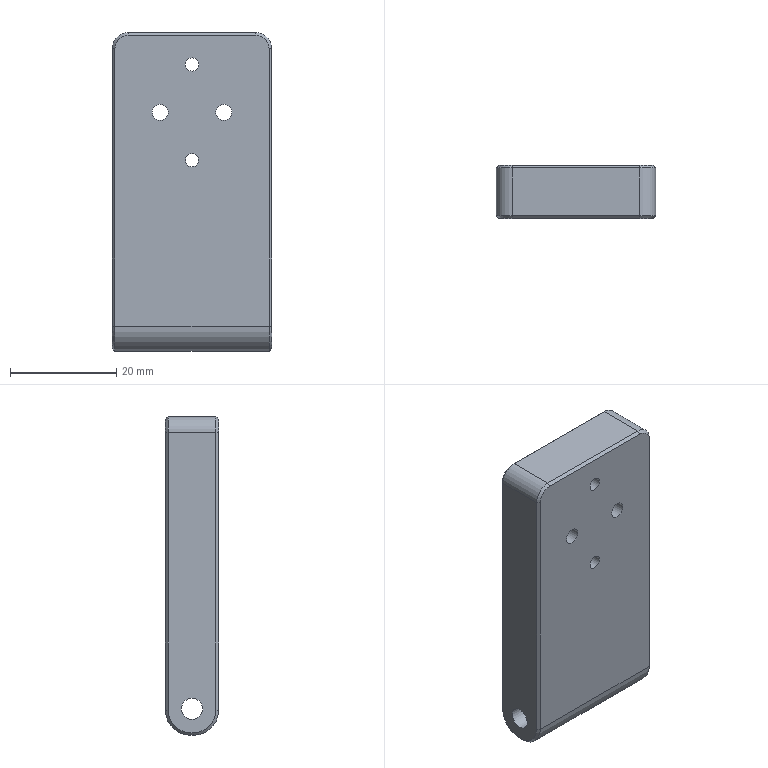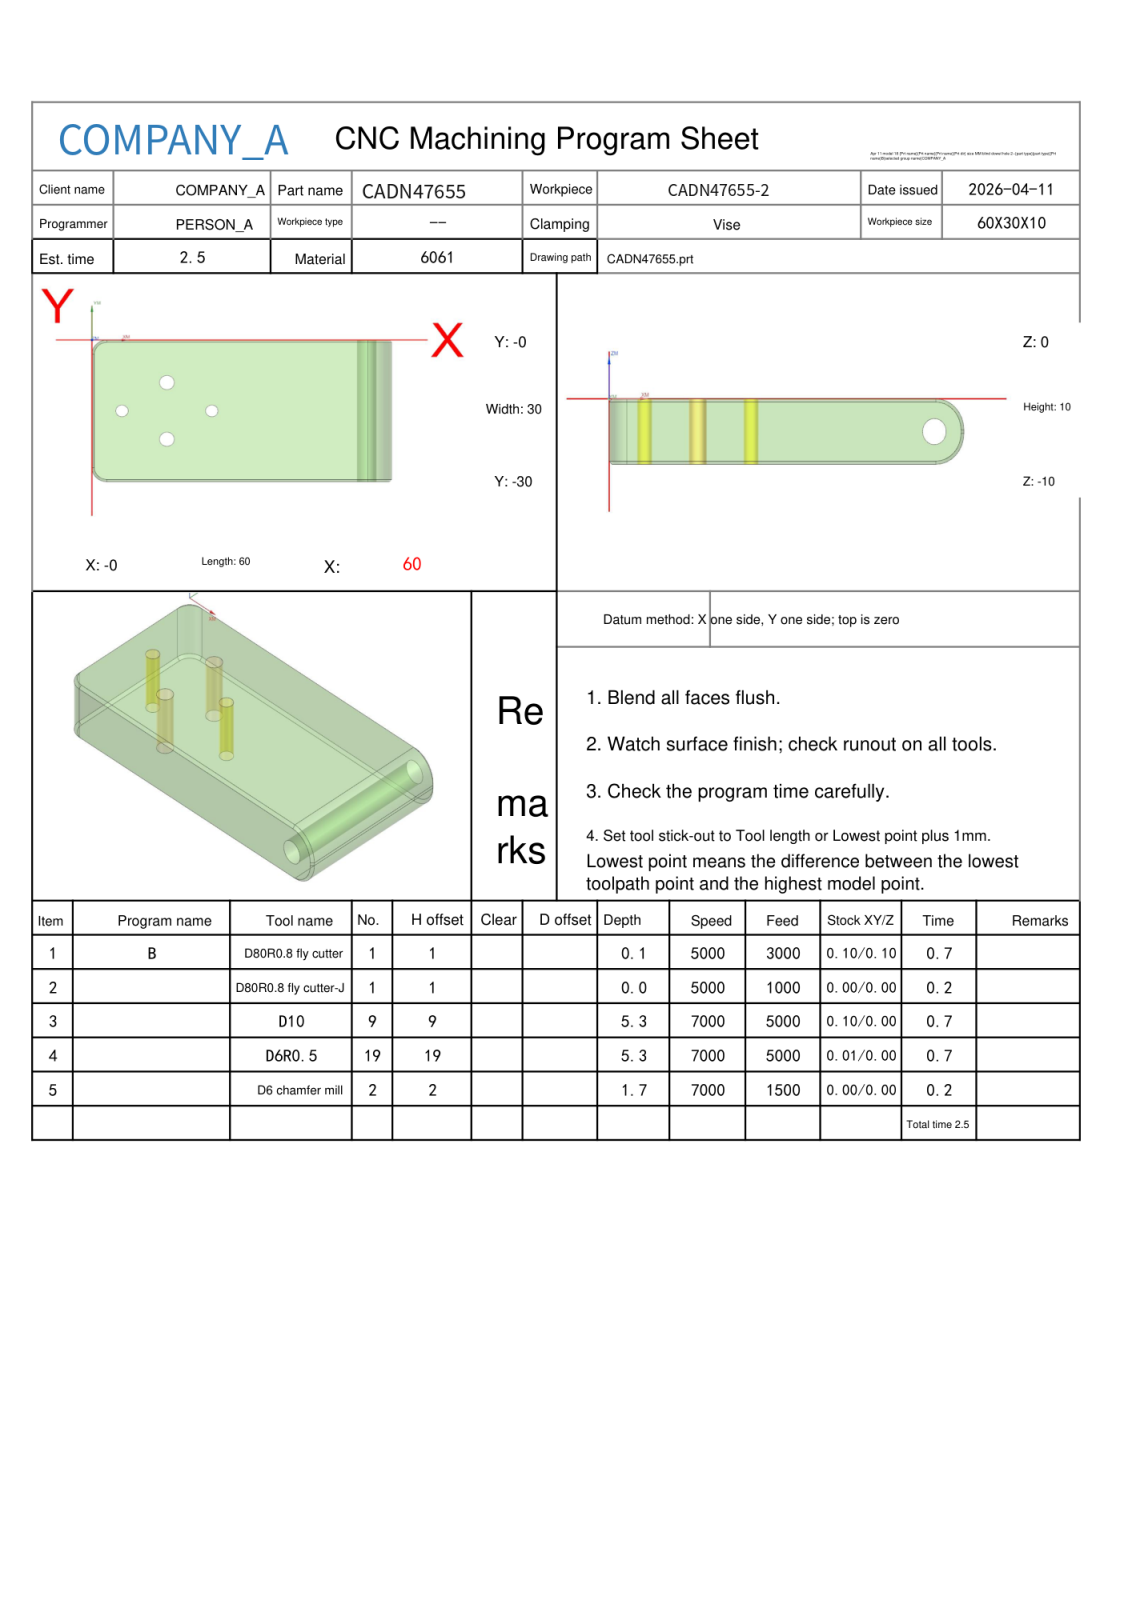NC program | NX | posted by the shop | part box 30 x 10 x 60 mm
Whole program, first 1498 of 1636 lines:
%
O0001
(Machine time: 3.37 MIN)
(===Total Tool:4===)
(T1=D80R0.8 fly cutter D=80.  R=0.8  D-  H01 Z=-0.   )
(T9=D10     D=10.  R=0.   D-  H09 Z=-5.35 )
(T19=D6R0.5 D=6.   R=0.5  D-  H19 Z=-5.35 )
(T2=D6 chamfer mill   D=6.   R=0.   D-  H02 Z=-1.75 )
G80 G90 G17 G49 G40
G91 G28 Z0
M01
N1 T01 M06
(D80R0.8 fly cutter  D=80. R=0.8 H=01 ce=0.10 di=0.10)
G00 G90 G54 X112.097 Y-15. M03 S5000
G43 H01 Z20.
M08
Z6.011
G01 Z4.011 F3000.
X100.097
X-40.097
X-52.097
Z6.011
G00 X112.097
Z5.522
G01 Z3.522
X100.097
X-40.097
X-52.097
Z5.522
G00 X112.097
Z5.033
G01 Z3.033
X100.097
X-40.097
X-52.097
Z5.033
G00 X112.097
Z4.544
G01 Z2.544
X100.097
X-40.097
X-52.097
Z4.544
G00 Z20.
X112.097
Z4.056
G01 Z2.056
X100.097
X-40.097
X-52.097
Z4.056
G00 Z20.
X112.097
Z3.567
G01 Z1.567
X100.097
X-40.097
X-52.097
Z3.567
G00 Z20.
X112.097
Z3.078
G01 Z1.078
X100.097
X-40.097
X-52.097
Z3.078
G00 Z20.
X112.097
Z2.589
G01 Z.589
X100.097
X-40.097
X-52.097
Z2.589
G00 Z20.
X112.097
Z2.1
G01 Z.1
X100.097
X-40.097
X-52.097
Z2.1
G00 Z20.
G91 G28 Z0.0
M05
M09
G91 G28 Z0.0
M01
N2 T01 M06
(D80R0.8 fly cutter-J  D=80. R=0.8 H=01 ce=0.00 di=0.00)
G00 G90 G54 X111.999 Y-14.998 M03 S5000
G43 H01 Z20.
M08
Z2.
G01 Z0.0 F1000.
X99.999 Y-14.999
X-39.999 Y-15.002
X-51.999
Z2.
G00 Z20.
G91 G28 Z0.0
M05
M09
G91 G28 Z0.0
M01
N3 T09 M06
(D10  D=10. R=0. H=09 ce=0.10 di=0.00)
G00 G90 G54 X48.978 Y9.606 M03 S7000
G43 H09 Z11.8
M08
Z.494
G01 Z-.006 F5000.
X48.983 Y9.445
G03 X53.98 Y4.604 I4.997 J.159
G01 X54.139 Y4.606
G02 X54.681 Y4.615 I.542 J-17.03
X56.195 Y4.548 I0.0 J-17.038
X60.598 Y-.5 I-.804 J-5.146
G01 Y-29.5
G02 X56.195 Y-34.548 I-5.208 J.098
X54.735 Y-34.618 I-1.46 J15.079
X54.139 Y-34.606 I0.0 J15.15
G01 X54.14 Y-34.614 Z-.014
G03 X54.692 Y-34.621 I.552 J22.478
X55.975 Y-34.584 I0.0 J22.485
X60.717 Y-29.5 I-.431 J5.155
G01 Y-.5
G03 X56.195 Y4.557 I-5.124 J-.031
X54.738 Y4.626 I-1.457 J-15.541
X54.14 Y4.614 I0.0 J-15.609
G01 Y4.624 Z-.024
G02 X54.724 Y4.632 I.584 J-21.478
X55.88 Y4.601 I0.0 J-21.485
X60.828 Y-.5 I-.243 J-5.186
G01 Y-29.5
G02 X55.976 Y-34.596 I-5.192 J.085
X54.688 Y-34.63 I-1.288 J23.89
X54.14 Y-34.624 I0.0 J23.925
G01 Y-34.636 Z-.036
G03 X54.7 Y-34.643 I.56 J21.788
X56.059 Y-34.601 I0.0 J21.795
X60.935 Y-29.5 I-.297 J5.165
G01 Y-.5
G03 X56.036 Y4.601 I-5.171 J-.063
X54.735 Y4.645 I-1.301 J-18.968
X54.14 Y4.636 I0.0 J-19.012
G01 Y4.65 Z-.05
G02 X54.742 Y4.66 I.602 J-18.398
X56.389 Y4.586 I0.0 J-18.408
X61.039 Y-.5 I-.457 J-5.086
G01 Y-29.5
G02 X56.195 Y-34.603 I-5.161 J.049
X54.715 Y-34.659 I-1.479 J19.52
X54.14 Y-34.65 I0.0 J19.576
G01 X54.141 Y-34.667 Z-.067
G03 X54.732 Y-34.677 I.591 J17.174
X56.588 Y-34.576 I0.0 J17.185
X61.142 Y-29.5 I-.551 J5.076
G01 Y-.5
G03 X56.64 Y4.567 I-5.154 J-.046
G01 X56.344 Y4.601
G03 X54.754 Y4.678 I-1.59 J-16.378
X54.141 Y4.667 I0.0 J-16.455
G01 Y4.685 Z-.085
G02 X54.768 Y4.697 I.626 J-15.524
X56.64 Y4.584 I0.0 J-15.536
X61.244 Y-.5 I-.562 J-5.135
G01 Y-29.5
G02 X56.64 Y-34.584 I-5.166 J.051
X54.753 Y-34.697 I-1.887 J15.791
X54.141 Y-34.685 I0.0 J15.903
G01 X54.142 Y-34.705 Z-.105
G03 X54.66 Y-34.709 I.518 J31.553
X55.75 Y-34.691 I0.0 J31.557
X57.606 Y-34.401 I-.349 J8.339
X61.344 Y-29.502 I-1.342 J4.9
G01 Y-.472
G03 X60.729 Y1.897 I-4.869 J0.0
X56.64 Y4.604 I-4.657 J-2.593
X54.77 Y4.718 I-1.87 J-15.236
X54.142 Y4.705 I0.0 J-15.35
G01 Y4.728 Z-.128
G02 X54.738 Y4.737 I.596 J-18.49
X56.195 Y4.68 I0.0 J-18.499
X58.419 Y4.157 I-.658 J-7.794
X61.444 Y-.5 I-2.142 J-4.702
G01 Y-29.5
G02 X57.084 Y-34.549 I-5.142 J.034
X54.782 Y-34.742 I-2.302 J13.584
X54.142 Y-34.728 I0.0 J13.777
G01 X54.143 Y-34.752 Z-.152
G03 X54.783 Y-34.767 I.64 J13.742
X56.914 Y-34.601 I0.0 J13.757
G01 X57.084 Y-34.572
X57.529 Y-34.483
G03 X61.542 Y-29.5 I-1.129 J5.017
G01 Y-.498
G03 X57.748 Y4.424 I-5.089 J0.0
X55.75 Y4.737 I-2.528 J-9.609
X54.718 Y4.759 I-1.032 J-24.001
X54.143 Y4.752 I0.0 J-24.023
G01 X54.144 Y4.779 Z-.179
X55.305 Y4.778
G02 X57.974 Y4.392 I-.124 J-10.256
X61.64 Y-.5 I-1.477 J-4.927
G01 Y-29.5
G02 X57.974 Y-34.392 I-5.143 J.035
G01 X57.794 Y-34.44
G02 X55.202 Y-34.778 I-2.595 J9.768
G01 X54.143 Y-34.779
X54.144 Y-34.807 Z-.207
X55.305
G03 X58.154 Y-34.362 I-.097 J9.96
X61.737 Y-29.502 I-1.505 J4.86
G01 Y-.5
G03 X58.16 Y4.36 I-5.09 J0.0
X55.75 Y4.791 I-2.92 J-9.382
X54.719 Y4.814 I-1.031 J-22.682
X54.144 Y4.807 I0.0 J-22.705
G01 X54.145 Y4.838 Z-.238
G02 X54.72 Y4.845 I.574 J-22.026
X55.75 Y4.821 I0.0 J-22.034
X58.441 Y4.294 I-.46 J-9.473
X61.834 Y-.498 I-1.688 J-4.792
G01 Y-29.503
G02 X58.315 Y-34.343 I-5.088 J0.0
X55.305 Y-34.837 I-3.131 J9.652
G01 X54.145 Y-34.838
Y-34.87 Z-.27
X55.305
G03 X58.559 Y-34.288 I-.102 J9.957
X61.929 Y-29.502 I-1.713 J4.786
G01 Y-.499
G03 X58.567 Y4.286 I-5.085 J0.0
X55.75 Y4.853 I-3.328 J-9.243
X54.72 Y4.878 I-1.03 J-21.336
X54.146 Y4.87 I0.0 J-21.36
G01 X54.147 Y4.905 Z-.305
G02 X54.729 Y4.914 I.582 J-18.707
X55.764 Y4.885 I0.0 J-18.716
X58.686 Y4.282 I-.559 J-10.094
X62.024 Y-.498 I-1.753 J-4.78
G01 Y-29.505
G02 X58.613 Y-34.309 I-5.089 J0.0
X55.104 Y-34.905 I-3.511 J10.056
G01 X54.146
X54.147 Y-34.941 Z-.341
X55.305
G03 X58.863 Y-34.253 I-.168 J10.412
X62.118 Y-29.5 I-1.886 J4.782
G01 Y-.5
G03 X58.863 Y4.253 I-5.14 J-.029
X56.195 Y4.893 I-3.842 J-10.141
X54.727 Y4.95 I-1.468 J-18.704
X54.148 Y4.941 I0.0 J-18.762
G01 X54.149 Y4.98 Z-.38
G02 X54.724 Y4.989 I.576 J-18.802
X56.195 Y4.931 I0.0 J-18.81
X58.863 Y4.289 I-1.197 J-10.845
X62.211 Y-.5 I-1.799 J-4.822
G01 Y-29.5
G02 X58.863 Y-34.289 I-5.146 J.033
X55.305 Y-34.979 I-3.734 J9.729
G01 X54.148 Y-34.98
X54.149 Y-35.02 Z-.42
X55.101
G03 X59.197 Y-34.189 I-.003 J10.526
X62.303 Y-29.503 I-1.981 J4.686
G01 Y-.497
G03 X59.225 Y4.177 I-5.088 J0.0
X55.644 Y5.006 I-4.086 J-9.502
X54.722 Y5.029 I-.922 J-18.84
X54.15 Y5.02 I0.0 J-18.862
G01 X54.152 Y5.062 Z-.462
G02 X54.641 Y5.068 I.489 J-22.187
X56.195 Y5.013 I0.0 J-22.193
X59.308 Y4.184 I-1.24 J-10.912
X62.394 Y-.5 I-2.05 J-4.709
G01 Y-29.5
G02 X59.308 Y-34.184 I-5.136 J.026
X56.195 Y-35.013 I-4.354 J10.084
X54.641 Y-35.068 I-1.554 J22.149
X54.152 Y-35.062 I0.0 J22.203
G01 X54.157 Y-35.085 Z-.485
X54.162 Y-35.106 Z-.507
G03 X54.628 Y-35.11 I.467 J23.01
X56.195 Y-35.057 I0.0 J23.015
X59.753 Y-34.015 I-1.22 J10.758
X62.485 Y-29.5 I-2.416 J4.546
G01 Y-.5
G03 X59.753 Y4.015 I-5.148 J-.031
X56.195 Y5.057 I-4.778 J-9.715
X54.611 Y5.111 I-1.584 J-23.31
X54.162 Y5.106 I0.0 J-23.364
G01 X54.163 Y5.129 Z-.53
X54.164 Y5.15 Z-.553
G02 X54.634 Y5.155 I.47 J-21.914
X56.195 Y5.1 I0.0 J-21.919
X59.753 Y4.06 I-1.224 J-10.799
X62.574 Y-.5 I-2.316 J-4.585
G01 Y-29.5
G02 X59.753 Y-34.06 I-5.137 J.025
X56.195 Y-35.099 I-4.782 J9.759
X54.657 Y-35.155 I-1.538 J21.308
X54.163 Y-35.149 I0.0 J21.363
G01 X54.164 Y-35.175 Z-.577
X54.165 Y-35.197 Z-.601
G03 X54.635 Y-35.202 I.47 J20.915
X56.195 Y-35.144 I0.0 J20.921
X59.928 Y-34.009 I-1.162 J10.529
X62.662 Y-29.501 I-2.349 J4.508
G01 Y-.497
G03 X59.959 Y3.994 I-5.081 J0.0
X55.638 Y5.178 I-4.812 J-9.084
X54.605 Y5.202 I-1.033 J-21.632
X54.166 Y5.198 I0.0 J-21.657
G01 X54.167 Y5.225 Z-.626
X54.168 Y5.247 Z-.65
G02 X54.575 Y5.251 I.407 J-21.392
X56.195 Y5.19 I0.0 J-21.396
X60.082 Y3.975 I-1.168 J-10.564
X62.749 Y-.499 I-2.419 J-4.474
G01 Y-29.501
G02 X60.082 Y-33.975 I-5.086 J0.0
X56.195 Y-35.19 I-5.054 J9.346
X54.613 Y-35.251 I-1.582 J20.422
X54.167 Y-35.246 I0.0 J20.483
G01 X54.168 Y-35.273 Z-.676
X54.169 Y-35.297 Z-.702
G03 X54.591 Y-35.301 I.423 J20.046
X55.655 Y-35.273 I0.0 J20.051
X60.325 Y-33.882 I-.552 J10.389
X62.835 Y-29.523 I-2.53 J4.359
G01 Y-.472
G03 X60.353 Y3.867 I-5.033 J0.0
X55.702 Y5.27 I-5.214 J-8.871
X54.544 Y5.302 I-1.157 J-21.104
X54.169 Y5.299 I0.0 J-21.136
G01 X54.171 Y5.328 Z-.729
X54.172 Y5.352 Z-.755
G02 X54.513 Y5.355 I.342 J-20.874
X55.769 Y5.317 I0.0 J-20.877
X59.918 Y4.15 I-.611 J-10.131
G01 X60.198 Y4.007
G02 X62.92 Y-.5 I-2.389 J-4.519
G01 Y-29.5
G02 X60.198 Y-34.007 I-5.112 J.012
G01 X59.766 Y-34.228
G02 X55.795 Y-35.316 I-4.603 J9.011
X54.57 Y-35.354 I-1.225 J19.587
X54.171 Y-35.35 I0.0 J19.626
G01 X54.172 Y-35.379 Z-.783
X54.173 Y-35.404 Z-.811
G03 X54.548 Y-35.408 I.375 J19.204
X55.805 Y-35.367 I0.0 J19.208
X59.762 Y-34.277 I-.665 J10.136
G01 X60.198 Y-34.054
G03 X63.004 Y-29.5 I-2.303 J4.561
G01 Y-.5
G03 X60.198 Y4.054 I-5.109 J-.007
G01 X60.009 Y4.15
G03 X55.76 Y5.369 I-4.884 J-9.009
X54.482 Y5.409 I-1.278 J-20.581
X54.174 Y5.407 I0.0 J-20.621
G01 X54.175 Y5.437 Z-.839
X54.176 Y5.463 Z-.867
G02 X54.45 Y5.465 I.274 J-20.366
X56.195 Y5.39 I0.0 J-20.368
X60.198 Y4.102 I-1.186 J-10.546
G01 X60.5 Y3.931
G02 X63.086 Y-.495 I-2.496 J-4.427
G01 Y-29.497
G02 X60.494 Y-33.935 I-5.094 J0.0
G01 X60.198 Y-34.102
G02 X56.195 Y-35.39 I-5.186 J9.254
X54.526 Y-35.464 I-1.668 J18.723
X54.175 Y-35.461 I0.0 J18.797
G01 X54.191 Y-35.519 Z-.926
G03 X54.616 Y-35.525 I.425 J14.224
X57.084 Y-35.309 I0.0 J14.23
X60.958 Y-33.7 I-2.338 J11.093
X63.168 Y-29.5 I-2.904 J4.209
G01 Y-.5
G03 X60.958 Y3.7 I-5.113 J-.009
X57.084 Y5.31 I-6.218 J-9.494
X54.575 Y5.527 I-2.51 J-14.406
X54.193 Y5.522 I0.0 J-14.623
G01 X54.237 Y5.582 Z-.986
G02 X54.58 Y5.586 I.343 J-14.294
X57.084 Y5.365 I0.0 J-14.298
X60.951 Y3.753 I-2.387 J-11.174
X63.248 Y-.493 I-2.777 J-4.246
G01 Y-29.508
G02 X60.952 Y-33.753 I-5.073 J0.0
X57.084 Y-35.364 I-6.249 J9.551
X54.609 Y-35.583 I-2.476 J13.88
X54.234 Y-35.578 I0.0 J14.099
G01 X54.279 Y-35.639 Z-1.048
G03 X54.615 Y-35.643 I.336 J13.803
X57.084 Y-35.421 I0.0 J13.807
X60.642 Y-33.997 I-2.388 J11.128
G01 X60.934 Y-33.815
G03 X63.327 Y-29.499 I-2.696 J4.316
G01 Y-.497
G03 X60.937 Y3.813 I-5.082 J0.0
G01 X60.642 Y3.997
G03 X57.084 Y5.421 I-5.953 J-9.715
X54.604 Y5.647 I-2.48 J-13.505
X54.282 Y5.643 I0.0 J-13.731
G01 X54.328 Y5.707 Z-1.112
G02 X54.672 Y5.711 I.345 J-12.45
X57.529 Y5.379 I0.0 J-12.455
X61.194 Y3.7 I-3.171 J-11.757
X63.404 Y-.5 I-2.902 J-4.208
G01 Y-29.5
G02 X61.194 Y-33.7 I-5.112 J.008
X57.529 Y-35.378 I-6.818 J10.046
X54.658 Y-35.706 I-2.871 J12.416
X54.325 Y-35.702 I0.0 J12.744
G01 X54.372 Y-35.765 Z-1.177
G03 X54.645 Y-35.768 I.273 J13.145
X57.084 Y-35.54 I0.0 J13.148
X61.532 Y-33.508 I-2.603 J11.58
X63.48 Y-29.5 I-3.167 J4.017
G01 Y-.5
G03 X61.532 Y3.508 I-5.115 J-.009
X57.529 Y5.438 I-7.159 J-9.727
X54.701 Y5.776 I-2.828 J-11.682
X54.375 Y5.771 I0.0 J-12.019
G01 X54.551 Y5.833 Z-1.244
G02 X54.881 Y5.838 I.33 J-10.415
X58.863 Y5.047 I0.0 J-10.421
G01 X59.143 Y4.928
G02 X61.087 Y3.866 I-4.43 J-10.422
G01 X61.217 Y3.783
G02 X63.555 Y-.495 I-2.744 J-4.278
G01 Y-29.5
G02 X61.346 Y-33.7 I-5.118 J.011
G01 X60.787 Y-34.058
G02 X57.084 Y-35.604 I-6.225 J9.703
X54.747 Y-35.828 I-2.338 J12.08
X54.499 Y-35.826 I0.0 J12.305
G01 X54.705 Y-35.838 Z-1.258
X54.91 Y-35.847 Z-1.271
X55.116 Y-35.856 Z-1.285
X55.322 Y-35.864 Z-1.299
X55.527 Y-35.861 Z-1.312
G03 X57.974 Y-35.434 I-.333 J9.13
X61.087 Y-33.917 I-3.909 J11.975
G01 X61.418 Y-33.7
G03 X63.628 Y-29.5 I-2.897 J4.206
G01 Y-.498
G03 X61.335 Y3.754 I-5.088 J0.0
G01 X61.087 Y3.917
G03 X59.126 Y4.99 I-6.424 J-9.411
G01 X58.982 Y5.052
X58.863 Y5.107
G03 X55.652 Y5.866 I-3.812 J-8.944
G01 X55.867 Z-1.326
X56.082 Y5.86 Z-1.34
X56.297 Y5.85 Z-1.354
X56.511 Y5.83 Z-1.368
X56.723 Y5.805 Z-1.382
G02 X58.48 Y5.322 I-1.474 J-8.797
X61.532 Y3.671 I-5.033 J-12.949
X63.7 Y-.5 I-2.945 J-4.179
G01 Y-29.5
G02 X61.532 Y-33.671 I-5.112 J.008
X58.419 Y-35.345 I-8.076 J11.289
X56.703 Y-35.805 I-3.253 J8.695
G01 X56.893 Y-35.79 Z-1.4
X57.083 Y-35.772 Z-1.418
X57.272 Y-35.746 Z-1.436
X57.458 Y-35.712 Z-1.454
G03 X58.419 Y-35.408 I-2.214 J8.654
X61.786 Y-33.533 I-5.004 J12.948
X63.77 Y-29.5 I-3.122 J4.04
G01 Y-.5
G03 X61.719 Y3.585 I-5.093 J0.0
X58.419 Y5.409 I-8.348 J-11.207
X57.457 Y5.711 I-2.883 J-7.498
G01 X57.64 Y5.686 Z-1.478
X57.821 Y5.655 Z-1.502
X58.002 Y5.622 Z-1.526
G02 X61.632 Y3.7 I-4.521 J-12.926
G01 X61.977 Y3.436
G02 X63.839 Y-.5 I-3.247 J-3.945
G01 Y-29.5
G02 X61.813 Y-33.567 I-5.116 J.011
G01 X61.632 Y-33.7
G02 X57.999 Y-35.622 I-8.146 J11.
G01 X58.21 Y-35.585 Z-1.563
X58.417 Y-35.538 Z-1.601
G03 X61.958 Y-33.504 I-5.321 J13.357
X63.906 Y-29.505 I-3.13 J3.998
G01 Y-.5
G03 X61.977 Y3.492 I-5.109 J-.007
X58.419 Y5.539 I-8.968 J-11.473
G01 X58.603 Y5.499 Z-1.638
X58.787 Y5.457 Z-1.676
G02 X61.977 Y3.539 I-6.175 J-13.886
X63.971 Y-.5 I-3.103 J-4.045
G01 Y-29.504
G02 X62.044 Y-33.487 I-5.078 J0.0
X58.785 Y-35.456 I-9.426 J11.916
G01 X58.939 Y-35.426 Z-1.715
X59.087 Y-35.381 Z-1.753
G03 X62.166 Y-33.436 I-6.578 J13.82
X64.035 Y-29.506 I-3.196 J3.93
G01 Y-.495
G03 X62.165 Y3.436 I-5.066 J0.0
X59.088 Y5.382 I-9.682 J-11.909
G01 X59.231 Y5.35 Z-1.792
X59.369 Y5.312 Z-1.832
G02 X62.224 Y3.442 I-7.609 J-14.728
X64.098 Y-.499 I-3.207 J-3.941
G01 Y-29.501
G02 X62.225 Y-33.441 I-5.08 J0.0
X59.368 Y-35.311 I-10.428 J12.808
G01 X59.498 Y-35.28 Z-1.871
X59.625 Y-35.242 Z-1.911
G03 X61.087 Y-34.336 I-8.598 J15.508
X61.977 Y-33.686 I-3.967 J6.368
X64.158 Y-29.5 I-2.956 J4.202
G01 Y-.5
G03 X61.977 Y3.686 I-5.137 J-.016
X61.087 Y4.336 I-4.876 J-5.743
X59.626 Y5.242 I-10.045 J-14.563
G01 X59.743 Y5.214 Z-1.952
X59.855 Y5.176 Z-1.992
G02 X61.532 Y4.083 I-13.184 J-22.071
G01 X62.281 Y3.493
G02 X64.217 Y-.495 I-3.141 J-3.989
G01 Y-29.5
G02 X62.253 Y-33.521 I-5.121 J.012
G01 X61.532 Y-34.083
G02 X59.854 Y-35.176 I-14.887 J21.034
G01 X60.057 Y-35.117 Z-2.074
G03 X60.845 Y-34.601 I-4.359 J7.516
X62.536 Y-33.328 I-7.992 J12.376
X64.275 Y-29.504 I-3.335 J3.824
G01 Y-.499
G03 X62.491 Y3.37 I-5.089 J0.0
X60.845 Y4.601 I-10.294 J-12.05
X60.058 Y5.117 I-5.099 J-6.92
G01 X60.263 Y5.058 Z-2.157
X61.211 Y4.405
G02 X62.609 Y3.314 I-8.496 J-12.323
X64.33 Y-.497 I-3.357 J-3.811
G01 Y-29.503
G02 X62.59 Y-33.33 I-5.08 J0.0
X61.174 Y-34.43 I-10.315 J11.819
G01 X60.262 Y-35.058
X60.425 Y-35.007 Z-2.242
X60.642 Y-34.86
X61.548 Y-34.214
G03 X62.303 Y-33.622 I-6.193 J8.672
G01 X62.736 Y-33.249
G03 X64.384 Y-29.5 I-3.461 J3.758
G01 Y-.498
G03 X62.617 Y3.351 I-5.077 J0.0
G01 X62.421 Y3.519
G03 X61.539 Y4.22 I-7.391 J-8.403
G01 X60.642 Y4.861
X60.427 Y5.007
X60.588 Y4.956 Z-2.327
G02 X62.866 Y3.18 I-11.998 J-17.74
X64.436 Y-.5 I-3.576 J-3.7
G01 Y-29.5
G02 X62.866 Y-33.18 I-5.146 J.02
X60.585 Y-34.957 I-14.21 J15.89
G01 X60.731 Y-34.913 Z-2.414
G03 X62.841 Y-33.249 I-13.622 J19.449
X64.486 Y-29.5 I-3.483 J3.763
G01 Y-.5
G03 X62.841 Y3.249 I-5.128 J-.014
X60.733 Y4.912 I-15.815 J-17.884
G01 X60.869 Y4.869 Z-2.502
G02 X62.866 Y3.272 I-15.328 J-21.221
X64.534 Y-.5 I-3.453 J-3.782
G01 Y-29.5
G02 X62.866 Y-33.272 I-5.121 J.01
X60.867 Y-34.869 I-17.278 J19.571
G01 X61.004 Y-34.824 Z-2.59
G03 X62.866 Y-33.313 I-17.071 J22.952
X64.581 Y-29.5 I-3.396 J3.819
G01 Y-.5
G03 X62.866 Y3.313 I-5.111 J-.006
X61.005 Y4.823 I-19.022 J-21.544
G01 X61.117 Y4.768 Z-2.635
X61.226 Y4.709 Z-2.68
G02 X62.941 Y3.283 I-17.516 J-22.809
X64.625 Y-.497 I-3.4 J-3.781
G01 Y-29.503
G02 X62.935 Y-33.289 I-5.085 J0.0
X61.13 Y-34.784 I-20.043 J22.355
G01 X61.236 Y-34.753 Z-2.77
X62.421 Y-33.788
X63.019 Y-33.249
X63.093 Y-33.185
G03 X64.668 Y-29.5 I-3.537 J3.691
G01 Y-.495
G03 X62.987 Y3.279 I-5.077 J0.0
G01 X62.421 Y3.788
X61.258 Y4.736
X61.277 Y4.751 Z-2.816
X61.286 Y4.759 Z-2.862
X62.421 Y3.828
X63.038 Y3.27
G02 X64.709 Y-.496 I-3.41 J-3.766
G01 Y-29.503
G02 X63.049 Y-33.258 I-5.076 J0.0
G01 X62.421 Y-33.828
X61.34 Y-34.715
X61.443 Y-34.677 Z-2.954
G03 X63.104 Y-33.249 I-21.975 J27.25
X64.747 Y-29.5 I-3.475 J3.758
G01 Y-.496
G03 X63.105 Y3.248 I-5.088 J0.0
X61.31 Y4.781 I-21.671 J-23.547
G01 X61.432 Y4.715 Z-3.001
X61.548 Y4.642 Z-3.047
X62.421 Y3.9
X63.142 Y3.249
G02 X64.784 Y-.5 I-3.476 J-3.757
G01 Y-29.501
G02 X63.205 Y-33.186 I-5.089 J0.0
X62.041 Y-34.218 I-14.777 J15.505
G01 X61.977 Y-34.271
X61.547 Y-34.642
X61.639 Y-34.61 Z-3.141
X61.977 Y-34.31
X62.06 Y-34.238
X62.102 Y-34.2
X62.124 Y-34.183
G03 X63.293 Y-33.132 I-11.665 J14.147
X64.819 Y-29.503 I-3.553 J3.63
G01 Y-.5
G03 X63.311 Y3.119 I-5.12 J-.009
X62.174 Y4.142 I-14.141 J-14.58
G02 X61.639 Y4.61 I9.501 J11.399
G01 X61.712 Y4.586 Z-3.235
G03 X62.143 Y4.203 I9.343 J10.074
G01 X62.179 Y4.173
G02 X63.439 Y3.024 I-12.166 J-14.596
X64.852 Y-.5 I-3.722 J-3.538
G01 Y-29.5
G02 X63.34 Y-33.12 I-5.106 J.007
X62.421 Y-33.971 I-16.903 J17.327
G01 X62.143 Y-34.203
G03 X61.836 Y-34.474 I6.348 J-7.497
G01 X61.848 Y-34.484 Z-3.283
X61.858 Y-34.492 Z-3.33
X62.162 Y-34.223
X62.648 Y-33.8
G03 X63.233 Y-33.249 I-6.664 J7.66
G01 X63.309 Y-33.185
G03 X64.883 Y-29.5 I-3.552 J3.696
G01 Y-.496
G03 X63.393 Y3.095 I-5.074 J0.0
X62.249 Y4.15 I-13.952 J-13.981
G01 X62.184 Y4.205
X61.777 Y4.566
X61.843 Y4.544 Z-3.426
X62.791 Y3.7
X63.262 Y3.249
X63.348 Y3.174
G02 X64.912 Y-.5 I-3.555 J-3.683
G01 Y-29.5
G02 X63.311 Y-33.209 I-5.109 J.005
G01 X63.262 Y-33.249
G02 X62.18 Y-34.242 I-15.505 J15.818
G01 X62.158 Y-34.259
X61.879 Y-34.51
X61.892 Y-34.521 Z-3.474
X61.9 Y-34.528 Z-3.523
X62.131 Y-34.312
G03 X63.415 Y-33.133 I-17.573 J20.415
X64.939 Y-29.505 I-3.556 J3.628
G01 Y-.49
G03 X63.449 Y3.099 I-5.069 J0.0
G01 X62.821 Y3.7
X61.977 Y4.455
X61.907 Y4.521
X61.971 Y4.497 Z-3.619
G03 X62.851 Y3.7 I16.616 J17.473
G01 X63.475 Y3.099
X63.548 Y3.024
G02 X64.963 Y-.5 I-3.689 J-3.528
G01 Y-29.509
G02 X63.318 Y-33.249 I-5.073 J0.0
X62.34 Y-34.15 I-10.48 J10.396
G01 X61.916 Y-34.546
X62.013 Y-34.486 Z-3.717
X62.421 Y-34.104
G03 X62.917 Y-33.661 I-4.571 J5.615
G01 X63.338 Y-33.249
X63.407 Y-33.185
G03 X64.986 Y-29.503 I-3.503 J3.682
G01 Y-29.5
Y-.5
G03 X63.499 Y3.099 I-5.111 J-.005
G01 X62.878 Y3.7
G02 X62.013 Y4.486 I15.5 J17.913
G01 X62.054 Y4.476 Z-3.815
G03 X62.901 Y3.7 I16.975 J17.68
G01 X63.437 Y3.174
X63.518 Y3.099
G02 X65.007 Y-.5 I-3.622 J-3.606
G01 Y-29.5
Y-29.502
G02 X63.425 Y-33.185 I-5.08 J0.0
G01 X63.358 Y-33.249
X62.983 Y-33.619
G02 X62.499 Y-34.065 I-6.653 J6.737
G03 X62.054 Y-34.476 I5.431 J-6.325
G01 X62.093 Y-34.466 Z-3.913
G02 X62.508 Y-34.077 I6.834 J-6.868
G03 X62.922 Y-33.692 I-7.851 J8.876
G01 X63.444 Y-33.185
G03 X65.026 Y-29.503 I-3.493 J3.682
G01 Y-29.5
Y-.495
G03 X63.501 Y3.13 I-5.073 J0.0
G01 X62.92 Y3.7
X62.248 Y4.314
X62.093 Y4.466
X62.13 Y4.452 Z-4.012
X62.262 Y4.327
X62.938 Y3.7
X63.515 Y3.135
G02 X65.042 Y-.496 I-3.553 J-3.631
G01 Y-29.502
G02 X63.552 Y-33.099 I-5.088 J0.0
X62.421 Y-34.173 I-21.352 J21.348
G01 X62.131 Y-34.453
X62.167 Y-34.438 Z-4.11
X62.212 Y-34.396
X62.464 Y-34.15
G03 X63.62 Y-33.042 I-15.592 J17.414
X65.057 Y-29.507 I-3.631 J3.535
G01 Y-.5
G03 X63.642 Y3.024 I-5.109 J-.005
G01 X63.569 Y3.099
X62.956 Y3.7
G02 X62.166 Y4.437 I18.172 J20.254
G01 X62.202 Y4.422 Z-4.21
X62.974 Y3.7
X63.567 Y3.111
G02 X65.069 Y-.494 I-3.577 J-3.606
G01 Y-29.51
G02 X63.559 Y-33.12 I-5.072 J0.0
G01 X62.974 Y-33.7
X62.301 Y-34.327
X62.204 Y-34.424
X62.235 Y-34.412 Z-4.309
X62.272 Y-34.378
X62.5 Y-34.15
G03 X63.628 Y-33.058 I-19.617 J21.401
X65.08 Y-29.502 I-3.633 J3.557
G01 Y-.5
G03 X63.515 Y3.174 I-5.119 J-.009
X62.233 Y4.41 I-52.57 J-53.243
G01 X62.254 Y4.405 Z-4.409
X63.311 Y3.385
X63.447 Y3.249
X63.67 Y3.024
G02 X65.088 Y-.5 I-3.703 J-3.537
G01 Y-29.499
G02 X63.635 Y-33.056 I-5.082 J0.0
G01 X63.447 Y-33.249
X63.311 Y-33.385
X62.255 Y-34.406
X62.275 Y-34.4 Z-4.509
X63.452 Y-33.249
X63.627 Y-33.072
G03 X65.094 Y-29.498 I-3.621 J3.574
G01 Y-.495
G03 X63.611 Y3.089 I-5.073 J0.0
X62.274 Y4.399 I-62.358 J-62.263
G01 X62.294 Y4.394 Z-4.609
X63.586 Y3.119
G02 X65.098 Y-.498 I-3.57 J-3.617
G01 Y-29.5
G02 X63.589 Y-33.12 I-5.118 J.009
G01 X62.54 Y-34.15
X62.295 Y-34.394
X62.312 Y-34.388 Z-4.708
X63.656 Y-33.056
G03 X65.099 Y-29.503 I-3.652 J3.553
G01 Y-29.5
Y-.487
G03 X63.537 Y3.174 I-5.096 J-.011
G01 X63.311 Y3.4
X62.314 Y4.388
X62.326 Y4.385 Z-4.808
X63.311 Y3.402
X63.622 Y3.089
G02 X65.099 Y-.49 I-3.597 J-3.58
G01 Y-29.5
Y-29.503
G02 X63.656 Y-33.056 I-5.095 J0.0
G01 X62.327 Y-34.384
Z-4.908
X63.656 Y-33.056
G03 X65.099 Y-29.503 I-3.652 J3.554
G01 Y-29.5
Y-.487
G03 X63.537 Y3.174 I-5.097 J-.011
G01 X62.421 Y4.291
X62.327 Y4.385
Z-5.008
X63.538 Y3.174
G02 X65.099 Y-.487 I-3.536 J-3.672
G01 Y-29.5
Y-29.502
G02 X63.656 Y-33.056 I-5.096 J0.0
G01 X62.327 Y-34.384
Z-5.093
X63.656 Y-33.056
G03 X65.1 Y-29.502 I-3.653 J3.554
G01 X65.099 Y-29.5
Y-.487
G03 X63.687 Y3.024 I-5.096 J-.011
G01 X63.614 Y3.099
X62.327 Y4.385
Z-5.179
X63.614 Y3.099
G02 X65.1 Y-.487 I-3.611 J-3.597
G01 Y-29.5
Y-29.502
G02 X63.656 Y-33.056 I-5.097 J0.0
G01 X62.327 Y-34.384
Z-5.264
X63.656 Y-33.056
G03 X65.1 Y-29.502 I-3.653 J3.554
G01 Y-29.5
Y-.487
G03 X63.614 Y3.099 I-5.097 J-.011
G01 X62.327 Y4.385
Z-5.35
X63.614 Y3.099
G02 X65.1 Y-.487 I-3.612 J-3.598
G01 Y-29.5
Y-29.501
G02 X63.656 Y-33.056 I-5.097 J0.0
G01 X62.327 Y-34.384
G00 Z11.8
G91 G28 Z0.0
M05
M09
G91 G28 Z0.0
M01
N4 T19 M06
(D6R0.5  D=6. R=0.5 H=19 ce=0.01 di=0.00)
G00 G90 G54 X51.218 Y5.088 M03 S7000
G43 H19 Z11.8
M08
Z.494
G01 Z-.006 F5000.
Y5.076
G03 X54.15 Y2.077 I3. J0.0
G02 X54.664 Y2.094 I.514 J-7.7
X56.225 Y1.934 I0.0 J-7.717
X58.014 Y-.5 I-.989 J-2.602
G01 Y-29.5
G02 X55.854 Y-31.992 I-2.617 J.086
X54.667 Y-32.096 I-1.187 J6.703
X54.15 Y-32.077 I0.0 J6.807
G01 X54.04 Y-32.12 Z-.013
G03 X54.644 Y-32.144 I.604 J7.535
X55.968 Y-32.027 I0.0 J7.559
X58.133 Y-29.5 I-.46 J2.585
G01 Y-.5
G03 X55.455 Y2.107 I-2.705 J-.1
G01 X54.037 Y2.121
X54.063 Y2.155 Z-.022
X55.534 Y2.142
G02 X58.245 Y-.5 I-.039 J-2.753
G01 Y-29.5
G02 X55.797 Y-32.115 I-2.721 J.094
G01 X55.534 Y-32.142
X54.062 Y-32.151
X54.09 Y-32.19 Z-.034
G03 X54.675 Y-32.208 I.585 J9.683
X55.983 Y-32.119 I0.0 J9.7
X58.353 Y-29.5 I-.37 J2.717
G01 Y-.5
G03 X55.949 Y2.122 I-2.739 J-.098
X54.632 Y2.203 I-1.317 J-10.702
X54.091 Y2.189 I0.0 J-10.783
G01 X54.112 Y2.216 Z-.047
X55.534 Y2.209
X55.88 Y2.177
G02 X58.458 Y-.5 I-.247 J-2.818
G01 Y-29.5
G02 X56.149 Y-32.125 I-2.732 J.075
X54.716 Y-32.236 I-1.433 J9.146
X54.108 Y-32.216 I0.0 J9.257
G01 X54.129 Y-32.246 Z-.062
X55.534 Y-32.238
X55.88 Y-32.209
G03 X58.561 Y-29.5 I-.175 J2.855
G01 Y-.5
G03 X55.88 Y2.209 I-2.856 J-.146
G01 X55.534 Y2.238
X54.136 Y2.247
X54.092 Y2.274 Z-.078
G02 X54.698 Y2.289 I.606 J-11.862
X56.225 Y2.191 I0.0 J-11.877
X58.663 Y-.5 I-.397 J-2.81
G01 Y-29.5
G02 X56.225 Y-32.191 I-2.835 J.119
X54.683 Y-32.289 I-1.542 J12.041
X54.086 Y-32.275 I0.0 J12.139
G01 X54.104 Y-32.299 Z-.097
X55.534 Y-32.294
G03 X57.346 Y-31.836 I-.065 J4.072
X58.765 Y-29.5 I-1.213 J2.336
G01 Y-.448
G03 X58.286 Y.99 I-2.397 J0.0
X55.88 Y2.273 I-2.574 J-1.93
G01 X55.534 Y2.294
X54.113 Y2.3
X54.136 Y2.329 Z-.118
X55.534 Y2.316
X55.88 Y2.297
G02 X58.309 Y1.105 I-.111 J-3.299
X58.865 Y-.435 I-1.856 J-1.54
G01 Y-29.5
G02 X57.262 Y-31.943 I-2.75 J.056
G01 X57.068 Y-32.021
G02 X55.561 Y-32.316 I-1.535 J3.841
G01 X54.124 Y-32.326
X54.146 Y-32.355 Z-.14
X55.534 Y-32.341
X55.545
G03 X57.262 Y-31.99 I0.0 J4.381
X58.964 Y-29.5 I-1.051 J2.545
G01 Y-.5
G03 X58.645 Y.749 I-2.997 J-.1
X56.225 Y2.286 I-2.728 J-1.621
X54.449 Y2.358 I-1.776 J-21.903
X54.141 Y2.356 I0.0 J-21.975
G01 X54.14 Y2.381 Z-.164
G02 X54.515 Y2.385 I.375 J-19.938
X56.225 Y2.311 I0.0 J-19.941
X58.743 Y.739 I-.228 J-3.166
X59.063 Y-.449 I-2.047 J-1.189
G01 Y-29.501
G02 X57.635 Y-31.868 I-2.674 J0.0
X55.88 Y-32.346 I-1.957 J3.716
G01 X55.534 Y-32.367
X54.147 Y-32.381
X54.123 Y-32.407 Z-.19
X55.534 Y-32.396
X55.88 Y-32.374
G03 X57.608 Y-31.943 I-.196 J4.465
X59.161 Y-29.5 I-1.218 J2.489
G01 Y-.5
G03 X57.94 Y1.746 I-2.677 J0.0
X56.225 Y2.339 I-2.055 J-3.169
X54.605 Y2.413 I-1.62 J-17.511
X54.149 Y2.407 I0.0 J-17.586
G01 X54.151 Y2.435 Z-.218
G02 X54.691 Y2.446 I.54 J-13.476
X56.571 Y2.314 I0.0 J-13.486
X58.721 Y1.092 I-.42 J-3.24
X59.258 Y-.462 I-1.979 J-1.554
G01 Y-29.5
G02 X57.608 Y-31.992 I-2.788 J.054
X55.88 Y-32.404 I-1.964 J4.404
G01 X55.534 Y-32.426
X54.132 Y-32.435
X54.141 Y-32.465 Z-.248
X55.649 Y-32.451
X55.88 Y-32.436
G03 X57.608 Y-32.044 I-.3 J5.335
X59.354 Y-29.5 I-1.068 J2.605
G01 Y-.467
G03 X58.81 Y1.103 I-2.535 J0.0
X56.763 Y2.313 I-2.588 J-2.041
X54.744 Y2.479 I-2.018 J-12.143
X54.151 Y2.465 I0.0 J-12.31
G01 Y2.497 Z-.28
G02 X54.689 Y2.504 I.538 J-19.763
X55.88 Y2.468 I0.0 J-19.771
X57.608 Y2.1 I-.472 J-6.45
X59.45 Y-.5 I-1.002 J-2.663
G01 Y-29.5
G02 X57.608 Y-32.1 I-2.844 J.063
X55.88 Y-32.468 I-2.2 J6.082
G01 X55.534 Y-32.489
X54.142 Y-32.497
X54.151 Y-32.53 Z-.313
X55.334 Y-32.523
G03 X57.616 Y-32.136 I-.041 J7.161
X59.545 Y-29.5 I-.927 J2.703
G01 Y-.5
G03 X57.617 Y2.135 I-2.856 J-.067
X55.65 Y2.514 I-2.317 J-6.745
X54.688 Y2.537 I-.962 J-19.601
X54.151 Y2.53 I0.0 J-19.625
G01 Y2.565 Z-.348
G02 X54.687 Y2.573 I.535 J-19.466
X55.88 Y2.536 I0.0 J-19.473
X57.954 Y2.039 I-.467 J-6.522
X59.64 Y-.5 I-1.152 J-2.594
G01 Y-29.5
G02 X57.954 Y-32.039 I-2.838 J.055
X55.409 Y-32.558 I-2.585 J6.179
G01 X54.151 Y-32.565
Y-32.602 Z-.385
X55.188
X55.221
G03 X57.954 Y-32.094 I0.0 J7.605
X59.733 Y-29.5 I-1.094 J2.659
G01 Y-.5
G03 X57.954 Y2.094 I-2.874 J-.064
X55.337 Y2.595 I-2.663 J-6.835
G01 X54.151 Y2.602
Y2.641 Z-.424
X55.264 Y2.633
G02 X57.977 Y2.127 I-.051 J-7.788
X59.826 Y-.5 I-1.018 J-2.681
G01 Y-29.5
G02 X57.954 Y-32.135 I-2.867 J.054
X55.206 Y-32.641 I-2.748 J7.215
G01 X55.188
X54.151
Y-32.681 Z-.464
X55.188
X55.196
G03 X57.954 Y-32.174 I0.0 J7.75
G01 X58.139 Y-32.105
G03 X59.918 Y-29.5 I-1.113 J2.67
G01 Y-.5
G03 X58.139 Y2.105 I-2.892 J-.065
G01 X57.954 Y2.174
G03 X55.318 Y2.673 I-2.687 J-6.983
G01 X54.151 Y2.681
Y2.723 Z-.506
G02 X54.681 Y2.731 I.53 J-18.812
X55.677 Y2.705 I0.0 J-18.82
X58.272 Y2.092 I-.396 J-7.479
X60.01 Y-.5 I-1.156 J-2.654
G01 Y-29.5
G02 X58.299 Y-32.08 I-2.894 J.062
X55.188 Y-32.723 I-3.129 J7.281
G01 X54.151
Y-32.767 Z-.55
X55.188
G03 X58.299 Y-32.127 I-.047 J8.11
X60.1 Y-29.5 I-1.101 J2.685
G01 Y-.5
G03 X58.299 Y2.127 I-2.902 J-.058
X55.88 Y2.736 I-3.222 J-7.689
X54.68 Y2.775 I-1.2 J-18.608
X54.151 Y2.767 I0.0 J-18.646
G01 X54.159 Y2.813 Z-.596
X55.534 Y2.802
G02 X58.645 Y2.003 I-.304 J-7.64
X60.189 Y-.5 I-1.321 J-2.543
G01 Y-29.5
G02 X58.645 Y-32.003 I-2.866 J.04
X55.534 Y-32.802 I-3.416 J6.842
G01 X54.159 Y-32.813
X54.154 Y-32.86 Z-.643
G03 X54.576 Y-32.864 I.422 J22.43
X55.514 Y-32.845 I0.0 J22.433
X58.648 Y-32.055 I-.332 J7.928
X60.278 Y-29.5 I-1.264 J2.604
G01 Y-.5
G03 X58.648 Y2.055 I-2.894 J-.049
X55.512 Y2.844 I-3.463 J-7.133
X54.566 Y2.864 I-.946 J-22.888
X54.154 Y2.86 I0.0 J-22.907
G01 X54.159 Y2.884 Z-.668
X54.164 Y2.909 Z-.692
G02 X54.599 Y2.914 I.435 J-17.161
X56.225 Y2.837 I0.0 J-17.167
X58.655 Y2.105 I-1.328 J-8.808
X60.365 Y-.5 I-1.221 J-2.665
G01 Y-29.5
G02 X58.655 Y-32.105 I-2.931 J.06
X55.88 Y-32.872 I-3.609 J7.657
X54.583 Y-32.912 I-1.296 J21.013
X54.163 Y-32.908 I0.0 J21.053
G01 X54.164 Y-32.933 Z-.717
X54.165 Y-32.958 Z-.743
X55.188 Y-32.955
G03 X58.991 Y-31.973 I-.061 J8.088
X60.452 Y-29.5 I-1.428 J2.512
G01 Y-.5
G03 X58.991 Y1.973 I-2.889 J-.04
X55.188 Y2.954 I-3.858 J-7.094
G01 X54.166 Y2.959
X54.167 Y2.985 Z-.769
Y3.011 Z-.795
X55.188 Y3.004
G02 X58.991 Y2.024 I-.07 J-8.14
X60.538 Y-.5 I-1.352 J-2.565
G01 Y-29.5
G02 X58.991 Y-32.024 I-2.899 J.041
X55.188 Y-33.005 I-3.88 J7.179
G01 X54.167 Y-33.01
X54.168 Y-33.036 Z-.822
X54.169 Y-33.063 Z-.849
G03 X54.507 Y-33.065 I.338 J23.991
X55.534 Y-33.043 I0.0 J23.993
X59.243 Y-31.926 I-.399 J8.038
X60.622 Y-29.503 I-1.438 J2.423
G01 Y-.497
G03 X59.243 Y1.926 I-2.817 J0.0
X55.88 Y3.018 I-4.101 J-6.909
X54.467 Y3.067 I-1.412 J-20.129
X54.169 Y3.065 I0.0 J-20.178
G01 X54.171 Y3.093 Z-.877
X54.172 Y3.12 Z-.904
G02 X54.508 Y3.124 I.336 J-15.933
X56.225 Y3.031 I0.0 J-15.937
X59.336 Y1.934 I-1.242 J-8.484
X60.706 Y-.5 I-1.564 J-2.482
G01 Y-29.5
G02 X59.336 Y-31.934 I-2.934 J.048
X55.188 Y-33.111 I-4.298 J7.252
G01 X54.171 Y-33.118
X54.172 Y-33.146 Z-.933
X54.173 Y-33.174 Z-.961
X55.188 Y-33.166
G03 X59.336 Y-31.985 I-.17 J8.471
X60.788 Y-29.5 I-1.464 J2.522
G01 Y-.5
G03 X59.336 Y1.985 I-2.916 J-.038
X56.225 Y3.083 I-4.356 J-7.385
X54.491 Y3.18 I-1.735 J-15.439
X54.174 Y3.177 I0.0 J-15.537
G01 X54.175 Y3.206 Z-.991
X54.176 Y3.235 Z-1.02
G02 X54.493 Y3.239 I.317 J-14.736
X55.819 Y3.179 I0.0 J-14.739
X59.581 Y1.878 I-.744 J-8.244
X60.87 Y-.495 I-1.54 J-2.373
G01 Y-29.501
G02 X59.566 Y-31.887 I-2.836 J0.0
X55.188 Y-33.222 I-4.554 J7.092
G01 X54.175 Y-33.232
X54.177 Y-33.262 Z-1.05
X54.178 Y-33.292 Z-1.08
G03 X54.438 Y-33.294 I.261 J18.038
X55.485 Y-33.263 I0.0 J18.04
X59.682 Y-31.873 I-.495 J8.526
X60.95 Y-29.5 I-1.656 J2.41
G01 Y-.5
G03 X59.682 Y1.873 I-2.923 J-.037
X55.721 Y3.246 I-4.687 J-7.122
X54.49 Y3.298 I-1.232 J-14.403
X54.178 Y3.295 I0.0 J-14.455
G01 X54.179 Y3.326 Z-1.111
X54.181 Y3.356 Z-1.142
G02 X54.416 Y3.358 I.235 J-17.241
X55.479 Y3.325 I0.0 J-17.243
X59.393 Y2.105 I-.531 J-8.593
G01 X59.682 Y1.935
G02 X61.029 Y-.5 I-1.61 J-2.48
G01 Y-29.5
G02 X59.682 Y-31.935 I-2.954 J.044
G01 X59.316 Y-32.151
G02 X55.458 Y-33.324 I-4.344 J7.359
X54.391 Y-33.354 I-1.067 J18.73
X54.18 Y-33.353 I0.0 J18.76
G01 X54.181 Y-33.384 Z-1.173
X54.183 Y-33.415 Z-1.205
X54.336 Y-33.416
G03 X55.88 Y-33.355 I0.0 J19.641
X59.881 Y-31.844 I-1.04 J8.806
X61.107 Y-29.507 I-1.615 J2.337
G01 Y-.5
G03 X60.004 Y1.76 I-2.942 J-.037
X56.225 Y3.313 I-5.249 J-7.395
X54.478 Y3.422 I-1.747 J-13.954
X54.183 Y3.419 I0.0 J-14.063
G01 X54.184 Y3.452 Z-1.237
X54.185 Y3.483 Z-1.269
G02 X54.472 Y3.486 I.287 J-13.863
X56.225 Y3.375 I0.0 J-13.866
X59.961 Y1.846 I-1.548 J-9.109
X61.183 Y-.497 I-1.633 J-2.343
G01 Y-29.503
G02 X59.962 Y-31.845 I-2.856 J0.0
X56.225 Y-33.372 I-5.26 J7.534
X54.443 Y-33.481 I-1.782 J14.524
X54.185 Y-33.479 I0.0 J14.633
G01 X54.346 Y-33.541 Z-1.335
X54.532 Y-33.543
G03 X56.225 Y-33.435 I0.0 J13.338
X59.682 Y-32.083 I-1.544 J9.045
G01 X60.028 Y-31.86
G03 X61.258 Y-29.5 I-1.712 J2.394
G01 Y-.5
G03 X60.028 Y1.86 I-2.943 J-.034
G01 X59.682 Y2.083
G03 X56.225 Y3.438 I-5.035 J-7.76
X54.593 Y3.549 I-1.632 J-11.974
X54.357 Y3.547 I0.0 J-12.085
G01 X54.478 Y3.568 Z-1.358
X54.598 Y3.589 Z-1.38
X54.719 Y3.608 Z-1.403
X54.908 Y3.61
G02 X57.76 Y3.09 I0.0 J-8.085
G01 X57.954 Y3.017
G02 X60.149 Y1.823 I-3.486 J-9.025
X61.332 Y-.497 I-1.683 J-2.32
G01 Y-29.502
G02 X60.151 Y-31.822 I-2.868 J0.0
X56.571 Y-33.438 I-5.682 J7.817
X54.803 Y-33.601 I-1.768 J9.495
G01 X54.66 Y-33.6
X54.817 Y-33.609 Z-1.414
X54.975 Y-33.617 Z-1.426
X55.132 Y-33.624 Z-1.437
X55.29 Y-33.632 Z-1.449
X55.448 Y-33.633 Z-1.46
X55.605 Y-33.632 Z-1.472
G03 X57.262 Y-33.323 I-.413 J6.818
X60.222 Y-31.828 I-3.112 J9.84
X61.405 Y-29.504 I-1.691 J2.324
G01 Y-.498
G03 X60.228 Y1.824 I-2.879 J0.0
X57.777 Y3.142 I-5.93 J-8.093
X55.672 Y3.636 I-2.67 J-6.637
G01 X55.816 Y3.638 Z-1.486
X55.96 Y3.637 Z-1.5
X56.104 Y3.632 Z-1.514
X56.247 Y3.62 Z-1.528
X56.389 Y3.605 Z-1.542
G02 X57.5 Y3.306 I-.981 J-5.848
G01 X57.767 Y3.205
G02 X60.392 Y1.76 I-3.717 J-9.859
X61.477 Y-.5 I-1.881 J-2.292
G01 Y-29.5
G02 X60.392 Y-31.76 I-2.965 J.033
X57.262 Y-33.389 I-6.481 J8.631
X56.374 Y-33.604 I-1.811 J5.519
G01 X56.546 Y-33.599 Z-1.566
X56.717 Y-33.587 Z-1.59
X56.884 Y-33.564 Z-1.614
G03 X60.373 Y-31.825 I-2.923 J10.234
X61.547 Y-29.5 I-1.761 J2.347
G01 Y-.5
G03 X60.373 Y1.825 I-2.934 J-.022
X56.889 Y3.564 I-6.432 J-8.527
G01 X57.015 Y3.552 Z-1.638
X57.14 Y3.538 Z-1.662
X57.264 Y3.524 Z-1.686
G02 X60.478 Y1.801 I-3.744 J-10.839
X61.615 Y-.499 I-1.755 J-2.299
G01 Y-29.501
G02 X60.478 Y-31.801 I-2.893 J0.0
X57.262 Y-33.524 I-6.948 J9.103
G01 X57.416 Y-33.51 Z-1.723
X57.566 Y-33.485 Z-1.761
G03 X60.373 Y-31.93 I-4.347 J11.157
G01 X60.602 Y-31.76
G03 X61.683 Y-29.5 I-1.889 J2.291
G01 Y-.5
G03 X60.602 Y1.76 I-2.969 J-.031
G01 X60.373 Y1.93
G03 X57.568 Y3.486 I-7.167 J-9.619
G01 X57.697 Y3.468 Z-1.798
X57.825 Y3.449 Z-1.836
G02 X60.719 Y1.721 I-4.934 J-11.553
X61.748 Y-.5 I-1.948 J-2.252
G01 Y-29.5
G02 X60.675 Y-31.76 I-2.981 J.031
X57.823 Y-33.449 I-7.855 J10.008
G01 X57.941 Y-33.436 Z-1.874
X58.056 Y-33.415 Z-1.913
G03 X60.686 Y-31.805 I-5.891 J12.579
X61.813 Y-29.504 I-1.788 J2.301
G01 Y-.496
G03 X60.686 Y1.805 I-2.914 J0.0
X58.057 Y3.415 I-8.545 J-11.
G01 X58.162 Y3.402 Z-1.952
X58.264 Y3.382 Z-1.99
G02 X60.809 Y1.76 I-6.445 J-12.917
X61.876 Y-.5 I-1.892 J-2.275
G01 Y-29.5
G02 X60.809 Y-31.76 I-2.959 J.015
X58.262 Y-33.382 I-8.966 J11.263
G01 X58.359 Y-33.368 Z-2.03
X58.454 Y-33.349 Z-2.07
G03 X60.827 Y-31.797 I-7.294 J13.749
X61.937 Y-29.501 I-1.82 J2.296
G01 Y-.499
G03 X60.827 Y1.797 I-2.93 J0.0
X58.455 Y3.349 I-9.697 J-12.235
G01 X58.552 Y3.337 Z-2.11
X58.646 Y3.319 Z-2.15
G02 X60.029 Y2.451 I-18.586 J-31.144
G01 X60.843 Y1.831
G02 X61.997 Y-.497 I-1.771 J-2.328
G01 Y-29.503
G02 X60.843 Y-31.832 I-2.926 J0.0
G01 X60.028 Y-32.451
G02 X58.645 Y-33.318 I-20.245 J30.75
G01 X58.79 Y-33.288 Z-2.231
G03 X60.095 Y-32.451 I-10.877 J18.388
G01 X60.912 Y-31.824
G03 X62.055 Y-29.506 I-1.779 J2.319
G01 Y-.5
G03 X60.996 Y1.76 I-2.972 J-.015
X58.791 Y3.288 I-11.03 J-13.554
G01 X58.942 Y3.264 Z-2.314
G02 X61.065 Y1.753 I-10.213 J-16.589
X62.112 Y-.5 I-1.933 J-2.268
G01 Y-29.5
G02 X61.065 Y-31.753 I-2.98 J.016
X58.941 Y-33.264 I-12.265 J14.988
G01 X59.077 Y-33.242 Z-2.397
G03 X61.112 Y-31.76 I-10.861 J17.053
X62.167 Y-29.5 I-1.927 J2.276
G01 Y-.5
G03 X61.112 Y1.76 I-2.983 J-.016
X59.078 Y3.242 I-12.979 J-15.674
G01 X59.206 Y3.218 Z-2.482
G02 X61.168 Y1.76 I-11.651 J-17.724
X62.221 Y-.5 I-1.927 J-2.273
G01 Y-29.5
G02 X61.168 Y-31.76 I-2.98 J.013
X59.204 Y-33.218 I-13.472 J16.086
G01 X59.334 Y-33.194 Z-2.567
X59.892 Y-32.796
X60.028 Y-32.696
X60.241 Y-32.543
G03 X61.065 Y-31.887 I-5.956 J8.32
G01 X61.224 Y-31.76
G03 X62.273 Y-29.5 I-1.947 J2.277
G01 Y-.496
G03 X61.165 Y1.807 I-2.947 J0.0
G01 X61.065 Y1.887
G03 X60.242 Y2.543 I-6.799 J-7.687
G01 X60.028 Y2.696
X59.893 Y2.796
X59.336 Y3.194
X59.448 Y3.172 Z-2.654
X60.373 Y2.493
X60.437 Y2.451
G02 X61.275 Y1.76 I-23.638 J-29.495
X62.323 Y-.5 I-1.942 J-2.274
G01 Y-29.5
G02 X61.275 Y-31.76 I-2.99 J.015
X60.437 Y-32.451 I-24.351 J28.655
G01 X60.373 Y-32.493
X59.491 Y-33.142
X59.447 Y-33.172
X59.562 Y-33.151 Z-2.741
X60.496 Y-32.451
X60.719 Y-32.274
X61.324 Y-31.76
G03 X62.372 Y-29.5 I-1.941 J2.272
G01 Y-.5
G03 X61.324 Y1.76 I-2.988 J-.013
G01 X60.719 Y2.274
X60.496 Y2.451
X59.563 Y3.151
X59.666 Y3.131 Z-2.829
X60.373 Y2.582
X60.551 Y2.451
X60.719 Y2.317
X61.41 Y1.726
G02 X62.419 Y-.5 I-1.982 J-2.239
G01 Y-29.5
G02 X61.374 Y-31.76 I-3.002 J.016
G01 X60.719 Y-32.317
X60.55 Y-32.451
X60.373 Y-32.582
X59.665 Y-33.132
X59.754 Y-33.117 Z-2.919
X60.604 Y-32.451
X60.719 Y-32.36
X61.41 Y-31.77
G03 X62.464 Y-29.5 I-1.959 J2.289
G01 Y-.5
G03 X61.41 Y1.77 I-3.012 J-.018
G01 X60.719 Y2.36
X59.755 Y3.116
X59.843 Y3.101 Z-3.009
X60.373 Y2.673
X60.659 Y2.451
G02 X61.756 Y1.475 I-7.993 J-10.092
X62.507 Y-.5 I-2.272 J-1.995
G01 Y-29.502
G02 X61.595 Y-31.634 I-2.948 J0.0
X60.659 Y-32.451 I-9.506 J9.955
G01 X60.373 Y-32.673
X59.842 Y-33.101
X59.93 Y-33.084 Z-3.099
X60.028 Y-33.003
X60.531 Y-32.598
G03 X61.616 Y-31.655 I-11.933 J14.836
X62.549 Y-29.502 I-2.017 J2.153
G01 Y-.498
G03 X61.621 Y1.651 I-2.95 J0.0
X60.558 Y2.576 I-12.488 J-13.273
G01 X60.028 Y3.003
X59.931 Y3.084
X60.017 Y3.064 Z-3.191
X60.373 Y2.765
X60.604 Y2.577
G02 X61.646 Y1.67 I-13.1 J-16.086
X62.589 Y-.499 I-2.021 J-2.169
G01 Y-29.5
G02 X61.756 Y-31.566 I-3.034 J.023
X60.719 Y-32.484 I-14.89 J15.788
G01 X60.373 Y-32.765
X60.016 Y-33.064
X60.085 Y-33.053 Z-3.283
G03 X61.675 Y-31.683 I-25.126 J30.761
X62.628 Y-29.5 I-2.069 J2.202
G01 Y-.5
G03 X61.756 Y1.607 I-3.035 J-.022
X60.086 Y3.053 I-25.361 J-27.605
G01 X60.152 Y3.043 Z-3.377
X60.719 Y2.558
X61.065 Y2.272
G02 X61.769 Y1.63 I-41.384 J-46.126
X62.664 Y-.5 I-2.137 J-2.151
G01 Y-29.5
G02 X61.756 Y-31.644 I-3.036 J.022
G01 X61.691 Y-31.699
G02 X61.065 Y-32.272 I-9.982 J10.27
G01 X60.719 Y-32.557
X60.152 Y-33.043
X60.219 Y-33.032 Z-3.47
X60.719 Y-32.595
X60.894 Y-32.451
G03 X61.93 Y-31.5 I-9.31 J11.196
X62.699 Y-29.5 I-2.294 J2.03
G01 Y-.5
G03 X61.93 Y1.5 I-3.063 J-.029
X60.894 Y2.451 I-10.171 J-10.052
G01 X60.719 Y2.595
X60.219 Y3.032
X60.283 Y3.018 Z-3.565
X60.719 Y2.632
X60.931 Y2.455
G02 X61.962 Y1.5 I-8.806 J-10.547
X62.732 Y-.5 I-2.298 J-2.033
G01 Y-29.5
G02 X61.924 Y-31.544 I-3.07 J.032
X61.065 Y-32.344 I-16.598 J16.971
G01 X60.719 Y-32.632
G02 X60.283 Y-33.018 I-26.676 J29.722
G01 X60.346 Y-33.002 Z-3.66
X60.373 Y-32.979
X60.719 Y-32.67
X60.84 Y-32.568
G03 X61.729 Y-31.76 I-10.366 J12.302
G01 X61.74 Y-31.747
G03 X62.763 Y-29.5 I-1.967 J2.252
G01 Y-.5
G03 X61.995 Y1.5 I-3.029 J-.016
X60.867 Y2.544 I-12.231 J-12.081
G02 X60.347 Y3.002 I12.038 J14.23
G01 X60.399 Y2.995 Z-3.755
G02 X61.9 Y1.63 I-31.55 J-36.22
X62.793 Y-.5 I-2.111 J-2.137
G01 Y-29.5
G02 X61.9 Y-31.63 I-3.003 J.007
X60.398 Y-32.995 I-33.073 J34.889
G01 X60.441 Y-32.993 Z-3.852
G03 X61.885 Y-31.673 I-49.873 J56.02
X62.82 Y-29.5 I-2.074 J2.181
G01 Y-.5
G03 X61.885 Y1.673 I-3.019 J-.012
X60.441 Y2.993 I-50.781 J-54.1
G01 X60.481 Y2.987 Z-3.948
G02 X61.918 Y1.666 I-41.307 J-46.359
X62.846 Y-.495 I-2.05 J-2.16
G01 Y-29.501
G02 X61.912 Y-31.671 I-2.99 J0.0
X60.481 Y-32.987 I-44.947 J47.457
G01 X60.519 Y-32.98 Z-4.045
G03 X61.957 Y-31.65 I-31.643 J35.633
X62.87 Y-29.5 I-2.073 J2.15
G01 Y-.5
G03 X61.98 Y1.63 I-3.02 J-.011
X60.519 Y2.98 I-35.493 J-36.927
G01 X60.558 Y2.973 Z-4.143
G02 X61.985 Y1.647 I-29.466 J-33.148
X62.892 Y-.498 I-2.082 J-2.145
G01 Y-29.5
G02 X62.005 Y-31.63 I-3.028 J.011
X60.558 Y-32.973 I-33.729 J34.886
G01 X60.597 Y-32.967 Z-4.241
G03 X61.065 Y-32.531 I-11.636 J12.953